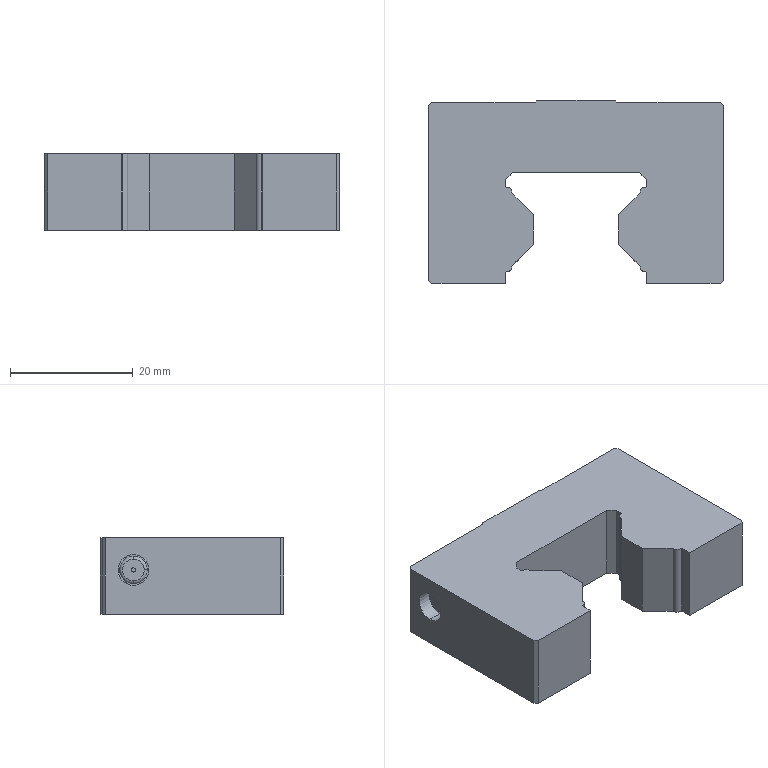Part | STEP file | 2026.6.15-Main Assembly图.sldasm-Part-54 | 1 solid | 63 faces | box 48 x 29.881 x 12.525 mm | volume 13643 mm3 | plane 39 | cylinder 18 | torus 6 | commonest cylinder face diameters 1.629 x8 5.01 x6 0.676 x4